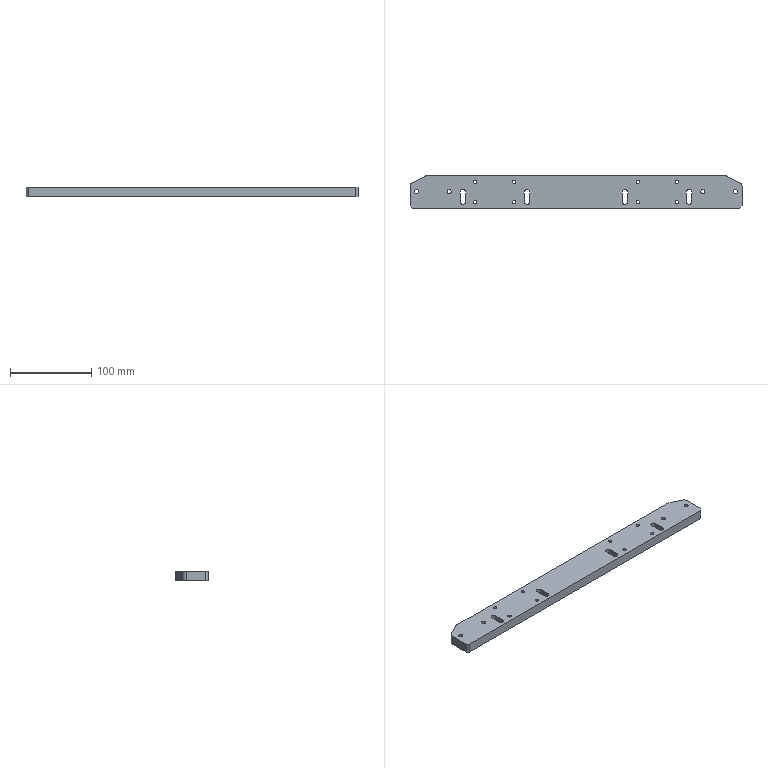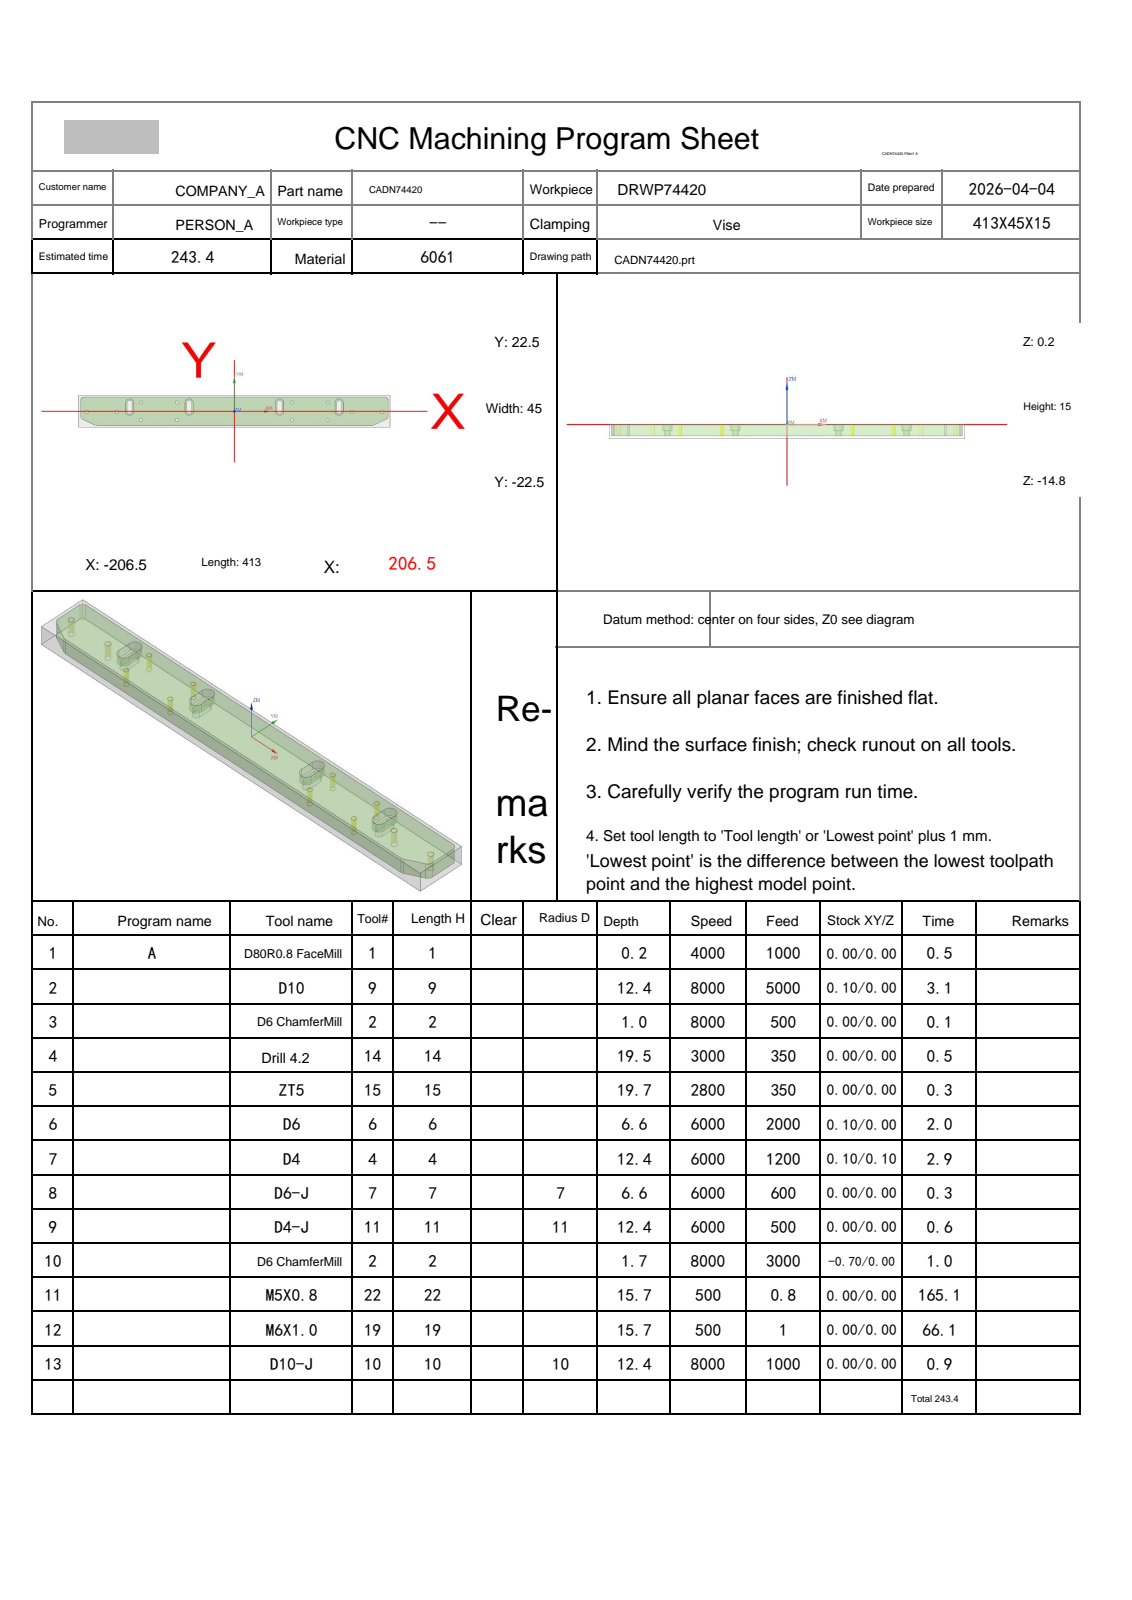NC program | NX | posted by the shop | part box 408 x 40 x 12 mm
Lines 1072 to 2398 of 2398:
N7 T04 M06
(D4  D=4. R=0. H=04 ce=0.10 di=0.10)
G00 G90 G54 X-140.2 Y6. M03 S6000
G43 H04 Z20.
M08
Z-5.9
G01 Y0.0 Z-5.946 F1200.
G03 X-139. Y-1.2 Z-5.961 I1.2 J0.0
X-137.8 Y0.0 Z-5.975 I0.0 J1.2
G01 Y12. Z-6.067
G03 X-139. Y13.2 Z-6.082 I-1.2 J0.0
X-140.2 Y12. Z-6.096 I0.0 J-1.2
G01 Y0.0 Z-6.188
G03 X-139. Y-1.2 Z-6.203 I1.2 J0.0
X-137.8 Y0.0 Z-6.217 I0.0 J1.2
G01 Y12. Z-6.31
G03 X-139. Y13.2 Z-6.324 I-1.2 J0.0
X-140.2 Y12. Z-6.339 I0.0 J-1.2
G01 Y0.0 Z-6.431
G03 X-139. Y-1.2 Z-6.445 I1.2 J0.0
X-137.8 Y0.0 Z-6.46 I0.0 J1.2
G01 Y12. Z-6.552
G03 X-139. Y13.2 Z-6.566 I-1.2 J0.0
X-140.2 Y12. Z-6.581 I0.0 J-1.2
G01 Y0.0 Z-6.673
G03 X-139. Y-1.2 Z-6.688 I1.2 J0.0
X-137.8 Y0.0 Z-6.702 I0.0 J1.2
G01 Y12. Z-6.794
G03 X-139. Y13.2 Z-6.809 I-1.2 J0.0
X-140.2 Y12. Z-6.823 I0.0 J-1.2
G01 Y0.0 Z-6.915
G03 X-139. Y-1.2 Z-6.93 I1.2 J0.0
X-137.8 Y0.0 Z-6.944 I0.0 J1.2
G01 Y12. Z-7.036
G03 X-139. Y13.2 Z-7.051 I-1.2 J0.0
X-140.2 Y12. Z-7.065 I0.0 J-1.2
G01 Y0.0 Z-7.158
G03 X-139. Y-1.2 Z-7.172 I1.2 J0.0
X-137.8 Y0.0 Z-7.187 I0.0 J1.2
G01 Y12. Z-7.279
G03 X-139. Y13.2 Z-7.293 I-1.2 J0.0
X-140.2 Y12. Z-7.308 I0.0 J-1.2
G01 Y0.0 Z-7.4
G03 X-139. Y-1.2 Z-7.414 I1.2 J0.0
X-137.8 Y0.0 Z-7.429 I0.0 J1.2
G01 Y12. Z-7.521
G03 X-139. Y13.2 Z-7.536 I-1.2 J0.0
X-140.2 Y12. Z-7.55 I0.0 J-1.2
G01 Y0.0 Z-7.642
G03 X-139. Y-1.2 Z-7.657 I1.2 J0.0
X-137.8 Y0.0 Z-7.671 I0.0 J1.2
G01 Y12. Z-7.763
G03 X-139. Y13.2 Z-7.778 I-1.2 J0.0
X-140.2 Y12. Z-7.792 I0.0 J-1.2
G01 Y0.0 Z-7.885
G03 X-139. Y-1.2 Z-7.899 I1.2 J0.0
X-137.8 Y0.0 Z-7.914 I0.0 J1.2
G01 Y12. Z-8.006
G03 X-139. Y13.2 Z-8.02 I-1.2 J0.0
X-140.2 Y12. Z-8.035 I0.0 J-1.2
G01 Y0.0 Z-8.127
G03 X-139. Y-1.2 Z-8.141 I1.2 J0.0
X-137.8 Y0.0 Z-8.156 I0.0 J1.2
G01 Y12. Z-8.248
G03 X-139. Y13.2 Z-8.263 I-1.2 J0.0
X-140.2 Y12. Z-8.277 I0.0 J-1.2
G01 Y0.0 Z-8.369
G03 X-139. Y-1.2 Z-8.384 I1.2 J0.0
X-137.8 Y0.0 Z-8.398 I0.0 J1.2
G01 Y12. Z-8.49
G03 X-139. Y13.2 Z-8.505 I-1.2 J0.0
X-140.2 Y12. Z-8.519 I0.0 J-1.2
G01 Y0.0 Z-8.611
G03 X-139. Y-1.2 Z-8.626 I1.2 J0.0
X-137.8 Y0.0 Z-8.64 I0.0 J1.2
G01 Y12. Z-8.733
G03 X-139. Y13.2 Z-8.747 I-1.2 J0.0
X-140.2 Y12. Z-8.762 I0.0 J-1.2
G01 Y0.0 Z-8.854
G03 X-139. Y-1.2 Z-8.868 I1.2 J0.0
X-137.8 Y0.0 Z-8.883 I0.0 J1.2
G01 Y12. Z-8.975
G03 X-139. Y13.2 Z-8.989 I-1.2 J0.0
X-140.2 Y12. Z-9.004 I0.0 J-1.2
G01 Y0.0 Z-9.096
G03 X-139. Y-1.2 Z-9.111 I1.2 J0.0
X-137.8 Y0.0 Z-9.125 I0.0 J1.2
G01 Y12. Z-9.217
G03 X-139. Y13.2 Z-9.232 I-1.2 J0.0
X-140.2 Y12. Z-9.246 I0.0 J-1.2
G01 Y0.0 Z-9.338
G03 X-139. Y-1.2 Z-9.353 I1.2 J0.0
X-137.8 Y0.0 Z-9.367 I0.0 J1.2
G01 Y12. Z-9.46
G03 X-139. Y13.2 Z-9.474 I-1.2 J0.0
X-140.2 Y12. Z-9.489 I0.0 J-1.2
G01 Y0.0 Z-9.581
G03 X-139. Y-1.2 Z-9.595 I1.2 J0.0
X-137.8 Y0.0 Z-9.61 I0.0 J1.2
G01 Y12. Z-9.702
G03 X-139. Y13.2 Z-9.716 I-1.2 J0.0
X-140.2 Y12. Z-9.731 I0.0 J-1.2
G01 Y0.0 Z-9.823
G03 X-139. Y-1.2 Z-9.838 I1.2 J0.0
X-137.8 Y0.0 Z-9.852 I0.0 J1.2
G01 Y12. Z-9.944
G03 X-139. Y13.2 Z-9.959 I-1.2 J0.0
X-140.2 Y12. Z-9.973 I0.0 J-1.2
G01 Y0.0 Z-10.065
G03 X-139. Y-1.2 Z-10.08 I1.2 J0.0
X-137.8 Y0.0 Z-10.094 I0.0 J1.2
G01 Y12. Z-10.186
G03 X-139. Y13.2 Z-10.201 I-1.2 J0.0
X-140.2 Y12. Z-10.215 I0.0 J-1.2
G01 Y0.0 Z-10.308
G03 X-139. Y-1.2 Z-10.322 I1.2 J0.0
X-137.8 Y0.0 Z-10.337 I0.0 J1.2
G01 Y12. Z-10.429
G03 X-139. Y13.2 Z-10.443 I-1.2 J0.0
X-140.2 Y12. Z-10.458 I0.0 J-1.2
G01 Y0.0 Z-10.55
G03 X-139. Y-1.2 Z-10.564 I1.2 J0.0
X-137.8 Y0.0 Z-10.579 I0.0 J1.2
G01 Y12. Z-10.671
G03 X-139. Y13.2 Z-10.686 I-1.2 J0.0
X-140.2 Y12. Z-10.7 I0.0 J-1.2
G01 Y0.0 Z-10.792
G03 X-139. Y-1.2 Z-10.807 I1.2 J0.0
X-137.8 Y0.0 Z-10.821 I0.0 J1.2
G01 Y12. Z-10.913
G03 X-139. Y13.2 Z-10.928 I-1.2 J0.0
X-140.2 Y12. Z-10.942 I0.0 J-1.2
G01 Y0.0 Z-11.035
G03 X-139. Y-1.2 Z-11.049 I1.2 J0.0
X-137.8 Y0.0 Z-11.064 I0.0 J1.2
G01 Y12. Z-11.156
G03 X-139. Y13.2 Z-11.17 I-1.2 J0.0
X-140.2 Y12. Z-11.185 I0.0 J-1.2
G01 Y0.0 Z-11.277
G03 X-139. Y-1.2 Z-11.291 I1.2 J0.0
X-137.8 Y0.0 Z-11.306 I0.0 J1.2
G01 Y12. Z-11.398
G03 X-139. Y13.2 Z-11.413 I-1.2 J0.0
X-140.2 Y12. Z-11.427 I0.0 J-1.2
G01 Y0.0 Z-11.519
G03 X-139. Y-1.2 Z-11.534 I1.2 J0.0
X-137.8 Y0.0 Z-11.548 I0.0 J1.2
G01 Y12. Z-11.64
G03 X-139. Y13.2 Z-11.655 I-1.2 J0.0
X-140.2 Y12. Z-11.669 I0.0 J-1.2
G01 Y0.0 Z-11.761
G03 X-139. Y-1.2 Z-11.776 I1.2 J0.0
X-137.8 Y0.0 Z-11.79 I0.0 J1.2
G01 Y12. Z-11.883
G03 X-139. Y13.2 Z-11.897 I-1.2 J0.0
X-140.2 Y12. Z-11.912 I0.0 J-1.2
G01 Y0.0 Z-12.004
G03 X-139. Y-1.2 Z-12.018 I1.2 J0.0
X-137.8 Y0.0 Z-12.033 I0.0 J1.2
G01 Y12. Z-12.125
G03 X-139. Y13.2 Z-12.139 I-1.2 J0.0
X-140.2 Y12. Z-12.154 I0.0 J-1.2
G01 Y6. Z-12.2
Y0.0
G03 X-139. Y-1.2 I1.2 J0.0
X-137.8 Y0.0 I0.0 J1.2
G01 Y12.
G03 X-139. Y13.2 I-1.2 J0.0
X-140.2 Y12. I0.0 J-1.2
G01 Y6.
Y5.5
Z-11.2
G00 Z20.
X-61.2 Y6.
Z-5.9
G01 Y0.0 Z-5.946
G03 X-60. Y-1.2 Z-5.961 I1.2 J0.0
X-58.8 Y0.0 Z-5.975 I0.0 J1.2
G01 Y12. Z-6.067
G03 X-59.28 Y12.96 Z-6.076 I-1.2 J0.0
X-60. Y13.2 Z-6.082 I-.72 J-.96
X-61.2 Y12. Z-6.096 I0.0 J-1.2
G01 Y0.0 Z-6.188
G03 X-60. Y-1.2 Z-6.203 I1.2 J0.0
X-58.8 Y0.0 Z-6.217 I0.0 J1.2
G01 Y12. Z-6.31
G03 X-59.28 Y12.96 Z-6.318 I-1.2 J0.0
X-60. Y13.2 Z-6.324 I-.72 J-.96
X-61.2 Y12. Z-6.339 I0.0 J-1.2
G01 Y0.0 Z-6.431
G03 X-60. Y-1.2 Z-6.445 I1.2 J0.0
X-58.8 Y0.0 Z-6.46 I0.0 J1.2
G01 Y12. Z-6.552
G03 X-59.28 Y12.96 Z-6.56 I-1.2 J0.0
X-60. Y13.2 Z-6.566 I-.72 J-.96
X-61.2 Y12. Z-6.581 I0.0 J-1.2
G01 Y0.0 Z-6.673
G03 X-60. Y-1.2 Z-6.688 I1.2 J0.0
X-58.8 Y0.0 Z-6.702 I0.0 J1.2
G01 Y12. Z-6.794
G03 X-59.28 Y12.96 Z-6.803 I-1.2 J0.0
X-60. Y13.2 Z-6.809 I-.72 J-.96
X-61.2 Y12. Z-6.823 I0.0 J-1.2
G01 Y0.0 Z-6.915
G03 X-60. Y-1.2 Z-6.93 I1.2 J0.0
X-58.8 Y0.0 Z-6.944 I0.0 J1.2
G01 Y12. Z-7.036
G03 X-59.28 Y12.96 Z-7.045 I-1.2 J0.0
X-60. Y13.2 Z-7.051 I-.72 J-.96
X-61.2 Y12. Z-7.065 I0.0 J-1.2
G01 Y0.0 Z-7.158
G03 X-60. Y-1.2 Z-7.172 I1.2 J0.0
X-58.8 Y0.0 Z-7.187 I0.0 J1.2
G01 Y12. Z-7.279
G03 X-59.28 Y12.96 Z-7.287 I-1.2 J0.0
X-60. Y13.2 Z-7.293 I-.72 J-.96
X-61.2 Y12. Z-7.308 I0.0 J-1.2
G01 Y0.0 Z-7.4
G03 X-60. Y-1.2 Z-7.414 I1.2 J0.0
X-58.8 Y0.0 Z-7.429 I0.0 J1.2
G01 Y12. Z-7.521
G03 X-59.28 Y12.96 Z-7.53 I-1.2 J0.0
X-60. Y13.2 Z-7.536 I-.72 J-.96
X-61.2 Y12. Z-7.55 I0.0 J-1.2
G01 Y0.0 Z-7.642
G03 X-60. Y-1.2 Z-7.657 I1.2 J0.0
X-58.8 Y0.0 Z-7.671 I0.0 J1.2
G01 Y12. Z-7.763
G03 X-59.28 Y12.96 Z-7.772 I-1.2 J0.0
X-60. Y13.2 Z-7.778 I-.72 J-.96
X-61.2 Y12. Z-7.792 I0.0 J-1.2
G01 Y0.0 Z-7.885
G03 X-60. Y-1.2 Z-7.899 I1.2 J0.0
X-58.8 Y0.0 Z-7.914 I0.0 J1.2
G01 Y12. Z-8.006
G03 X-59.28 Y12.96 Z-8.014 I-1.2 J0.0
X-60. Y13.2 Z-8.02 I-.72 J-.96
X-61.2 Y12. Z-8.035 I0.0 J-1.2
G01 Y0.0 Z-8.127
G03 X-60. Y-1.2 Z-8.141 I1.2 J0.0
X-58.8 Y0.0 Z-8.156 I0.0 J1.2
G01 Y12. Z-8.248
G03 X-59.28 Y12.96 Z-8.257 I-1.2 J0.0
X-60. Y13.2 Z-8.263 I-.72 J-.96
X-61.2 Y12. Z-8.277 I0.0 J-1.2
G01 Y0.0 Z-8.369
G03 X-60. Y-1.2 Z-8.384 I1.2 J0.0
X-58.8 Y0.0 Z-8.398 I0.0 J1.2
G01 Y12. Z-8.49
G03 X-59.28 Y12.96 Z-8.499 I-1.2 J0.0
X-60. Y13.2 Z-8.505 I-.72 J-.96
X-61.2 Y12. Z-8.519 I0.0 J-1.2
G01 Y0.0 Z-8.611
G03 X-60. Y-1.2 Z-8.626 I1.2 J0.0
X-58.8 Y0.0 Z-8.64 I0.0 J1.2
G01 Y12. Z-8.733
G03 X-59.28 Y12.96 Z-8.741 I-1.2 J0.0
X-60. Y13.2 Z-8.747 I-.72 J-.96
X-61.2 Y12. Z-8.762 I0.0 J-1.2
G01 Y0.0 Z-8.854
G03 X-60. Y-1.2 Z-8.868 I1.2 J0.0
X-58.8 Y0.0 Z-8.883 I0.0 J1.2
G01 Y12. Z-8.975
G03 X-59.28 Y12.96 Z-8.983 I-1.2 J0.0
X-60. Y13.2 Z-8.989 I-.72 J-.96
X-61.2 Y12. Z-9.004 I0.0 J-1.2
G01 Y0.0 Z-9.096
G03 X-60. Y-1.2 Z-9.111 I1.2 J0.0
X-58.8 Y0.0 Z-9.125 I0.0 J1.2
G01 Y12. Z-9.217
G03 X-59.28 Y12.96 Z-9.226 I-1.2 J0.0
X-60. Y13.2 Z-9.232 I-.72 J-.96
X-61.2 Y12. Z-9.246 I0.0 J-1.2
G01 Y0.0 Z-9.338
G03 X-60. Y-1.2 Z-9.353 I1.2 J0.0
X-58.8 Y0.0 Z-9.367 I0.0 J1.2
G01 Y12. Z-9.46
G03 X-59.28 Y12.96 Z-9.468 I-1.2 J0.0
X-60. Y13.2 Z-9.474 I-.72 J-.96
X-61.2 Y12. Z-9.489 I0.0 J-1.2
G01 Y0.0 Z-9.581
G03 X-60. Y-1.2 Z-9.595 I1.2 J0.0
X-58.8 Y0.0 Z-9.61 I0.0 J1.2
G01 Y12. Z-9.702
G03 X-59.28 Y12.96 Z-9.71 I-1.2 J0.0
X-60. Y13.2 Z-9.716 I-.72 J-.96
X-61.2 Y12. Z-9.731 I0.0 J-1.2
G01 Y0.0 Z-9.823
G03 X-60. Y-1.2 Z-9.838 I1.2 J0.0
X-58.8 Y0.0 Z-9.852 I0.0 J1.2
G01 Y12. Z-9.944
G03 X-59.28 Y12.96 Z-9.953 I-1.2 J0.0
X-60. Y13.2 Z-9.959 I-.72 J-.96
X-61.2 Y12. Z-9.973 I0.0 J-1.2
G01 Y0.0 Z-10.065
G03 X-60. Y-1.2 Z-10.08 I1.2 J0.0
X-58.8 Y0.0 Z-10.094 I0.0 J1.2
G01 Y12. Z-10.186
G03 X-59.28 Y12.96 Z-10.195 I-1.2 J0.0
X-60. Y13.2 Z-10.201 I-.72 J-.96
X-61.2 Y12. Z-10.215 I0.0 J-1.2
G01 Y0.0 Z-10.308
G03 X-60. Y-1.2 Z-10.322 I1.2 J0.0
X-58.8 Y0.0 Z-10.337 I0.0 J1.2
G01 Y12. Z-10.429
G03 X-59.28 Y12.96 Z-10.437 I-1.2 J0.0
X-60. Y13.2 Z-10.443 I-.72 J-.96
X-61.2 Y12. Z-10.458 I0.0 J-1.2
G01 Y0.0 Z-10.55
G03 X-60. Y-1.2 Z-10.564 I1.2 J0.0
X-58.8 Y0.0 Z-10.579 I0.0 J1.2
G01 Y12. Z-10.671
G03 X-59.28 Y12.96 Z-10.68 I-1.2 J0.0
X-60. Y13.2 Z-10.686 I-.72 J-.96
X-61.2 Y12. Z-10.7 I0.0 J-1.2
G01 Y0.0 Z-10.792
G03 X-60. Y-1.2 Z-10.807 I1.2 J0.0
X-58.8 Y0.0 Z-10.821 I0.0 J1.2
G01 Y12. Z-10.913
G03 X-59.28 Y12.96 Z-10.922 I-1.2 J0.0
X-60. Y13.2 Z-10.928 I-.72 J-.96
X-61.2 Y12. Z-10.942 I0.0 J-1.2
G01 Y0.0 Z-11.035
G03 X-60. Y-1.2 Z-11.049 I1.2 J0.0
X-58.8 Y0.0 Z-11.064 I0.0 J1.2
G01 Y12. Z-11.156
G03 X-59.28 Y12.96 Z-11.164 I-1.2 J0.0
X-60. Y13.2 Z-11.17 I-.72 J-.96
X-61.2 Y12. Z-11.185 I0.0 J-1.2
G01 Y0.0 Z-11.277
G03 X-60. Y-1.2 Z-11.291 I1.2 J0.0
X-58.8 Y0.0 Z-11.306 I0.0 J1.2
G01 Y12. Z-11.398
G03 X-59.28 Y12.96 Z-11.407 I-1.2 J0.0
X-60. Y13.2 Z-11.413 I-.72 J-.96
X-61.2 Y12. Z-11.427 I0.0 J-1.2
G01 Y0.0 Z-11.519
G03 X-60. Y-1.2 Z-11.534 I1.2 J0.0
X-58.8 Y0.0 Z-11.548 I0.0 J1.2
G01 Y12. Z-11.64
G03 X-59.28 Y12.96 Z-11.649 I-1.2 J0.0
X-60. Y13.2 Z-11.655 I-.72 J-.96
X-61.2 Y12. Z-11.669 I0.0 J-1.2
G01 Y0.0 Z-11.761
G03 X-60. Y-1.2 Z-11.776 I1.2 J0.0
X-58.8 Y0.0 Z-11.79 I0.0 J1.2
G01 Y12. Z-11.883
G03 X-59.28 Y12.96 Z-11.891 I-1.2 J0.0
X-60. Y13.2 Z-11.897 I-.72 J-.96
X-61.2 Y12. Z-11.912 I0.0 J-1.2
G01 Y0.0 Z-12.004
G03 X-60. Y-1.2 Z-12.018 I1.2 J0.0
X-58.8 Y0.0 Z-12.033 I0.0 J1.2
G01 Y12. Z-12.125
G03 X-59.28 Y12.96 Z-12.133 I-1.2 J0.0
X-60. Y13.2 Z-12.139 I-.72 J-.96
X-61.2 Y12. Z-12.154 I0.0 J-1.2
G01 Y6. Z-12.2
Y0.0
G03 X-60. Y-1.2 I1.2 J0.0
X-58.8 Y0.0 I0.0 J1.2
G01 Y12.
G03 X-60. Y13.2 I-1.2 J0.0
X-61.2 Y12. I0.0 J-1.2
G01 Y6.
Y5.5
Z-11.2
G00 Z20.
X58.8 Y6.
Z-5.9
G01 Y0.0 Z-5.946
G03 X60. Y-1.2 Z-5.961 I1.2 J0.0
X61.2 Y0.0 Z-5.975 I0.0 J1.2
G01 Y12. Z-6.067
G03 X60. Y13.2 Z-6.082 I-1.2 J0.0
X59.316 Y12.986 Z-6.087 I0.0 J-1.2
X58.8 Y12. Z-6.096 I.684 J-.986
G01 Y0.0 Z-6.188
G03 X60. Y-1.2 Z-6.203 I1.2 J0.0
X61.2 Y0.0 Z-6.217 I0.0 J1.2
G01 Y12. Z-6.31
G03 X60. Y13.2 Z-6.324 I-1.2 J0.0
X59.316 Y12.986 Z-6.33 I0.0 J-1.2
X58.8 Y12. Z-6.339 I.684 J-.986
G01 Y0.0 Z-6.431
G03 X60. Y-1.2 Z-6.445 I1.2 J0.0
X61.2 Y0.0 Z-6.46 I0.0 J1.2
G01 Y12. Z-6.552
G03 X60. Y13.2 Z-6.566 I-1.2 J0.0
X59.316 Y12.986 Z-6.572 I0.0 J-1.2
X58.8 Y12. Z-6.581 I.684 J-.986
G01 Y0.0 Z-6.673
G03 X60. Y-1.2 Z-6.688 I1.2 J0.0
X61.2 Y0.0 Z-6.702 I0.0 J1.2
G01 Y12. Z-6.794
G03 X60. Y13.2 Z-6.809 I-1.2 J0.0
X59.316 Y12.986 Z-6.814 I0.0 J-1.2
X58.8 Y12. Z-6.823 I.684 J-.986
G01 Y0.0 Z-6.915
G03 X60. Y-1.2 Z-6.93 I1.2 J0.0
X61.2 Y0.0 Z-6.944 I0.0 J1.2
G01 Y12. Z-7.036
G03 X60. Y13.2 Z-7.051 I-1.2 J0.0
X59.316 Y12.986 Z-7.057 I0.0 J-1.2
X58.8 Y12. Z-7.065 I.684 J-.986
G01 Y0.0 Z-7.158
G03 X60. Y-1.2 Z-7.172 I1.2 J0.0
X61.2 Y0.0 Z-7.187 I0.0 J1.2
G01 Y12. Z-7.279
G03 X60. Y13.2 Z-7.293 I-1.2 J0.0
X59.316 Y12.986 Z-7.299 I0.0 J-1.2
X58.8 Y12. Z-7.308 I.684 J-.986
G01 Y0.0 Z-7.4
G03 X60. Y-1.2 Z-7.414 I1.2 J0.0
X61.2 Y0.0 Z-7.429 I0.0 J1.2
G01 Y12. Z-7.521
G03 X60. Y13.2 Z-7.536 I-1.2 J0.0
X59.316 Y12.986 Z-7.541 I0.0 J-1.2
X58.8 Y12. Z-7.55 I.684 J-.986
G01 Y0.0 Z-7.642
G03 X60. Y-1.2 Z-7.657 I1.2 J0.0
X61.2 Y0.0 Z-7.671 I0.0 J1.2
G01 Y12. Z-7.763
G03 X60. Y13.2 Z-7.778 I-1.2 J0.0
X59.316 Y12.986 Z-7.783 I0.0 J-1.2
X58.8 Y12. Z-7.792 I.684 J-.986
G01 Y0.0 Z-7.885
G03 X60. Y-1.2 Z-7.899 I1.2 J0.0
X61.2 Y0.0 Z-7.914 I0.0 J1.2
G01 Y12. Z-8.006
G03 X60. Y13.2 Z-8.02 I-1.2 J0.0
X59.316 Y12.986 Z-8.026 I0.0 J-1.2
X58.8 Y12. Z-8.035 I.684 J-.986
G01 Y0.0 Z-8.127
G03 X60. Y-1.2 Z-8.141 I1.2 J0.0
X61.2 Y0.0 Z-8.156 I0.0 J1.2
G01 Y12. Z-8.248
G03 X60. Y13.2 Z-8.263 I-1.2 J0.0
X59.316 Y12.986 Z-8.268 I0.0 J-1.2
X58.8 Y12. Z-8.277 I.684 J-.986
G01 Y0.0 Z-8.369
G03 X60. Y-1.2 Z-8.384 I1.2 J0.0
X61.2 Y0.0 Z-8.398 I0.0 J1.2
G01 Y12. Z-8.49
G03 X60. Y13.2 Z-8.505 I-1.2 J0.0
X59.316 Y12.986 Z-8.51 I0.0 J-1.2
X58.8 Y12. Z-8.519 I.684 J-.986
G01 Y0.0 Z-8.611
G03 X60. Y-1.2 Z-8.626 I1.2 J0.0
X61.2 Y0.0 Z-8.64 I0.0 J1.2
G01 Y12. Z-8.733
G03 X60. Y13.2 Z-8.747 I-1.2 J0.0
X59.316 Y12.986 Z-8.753 I0.0 J-1.2
X58.8 Y12. Z-8.762 I.684 J-.986
G01 Y0.0 Z-8.854
G03 X60. Y-1.2 Z-8.868 I1.2 J0.0
X61.2 Y0.0 Z-8.883 I0.0 J1.2
G01 Y12. Z-8.975
G03 X60. Y13.2 Z-8.989 I-1.2 J0.0
X59.316 Y12.986 Z-8.995 I0.0 J-1.2
X58.8 Y12. Z-9.004 I.684 J-.986
G01 Y0.0 Z-9.096
G03 X60. Y-1.2 Z-9.111 I1.2 J0.0
X61.2 Y0.0 Z-9.125 I0.0 J1.2
G01 Y12. Z-9.217
G03 X60. Y13.2 Z-9.232 I-1.2 J0.0
X59.316 Y12.986 Z-9.237 I0.0 J-1.2
X58.8 Y12. Z-9.246 I.684 J-.986
G01 Y0.0 Z-9.338
G03 X60. Y-1.2 Z-9.353 I1.2 J0.0
X61.2 Y0.0 Z-9.367 I0.0 J1.2
G01 Y12. Z-9.46
G03 X60. Y13.2 Z-9.474 I-1.2 J0.0
X59.316 Y12.986 Z-9.48 I0.0 J-1.2
X58.8 Y12. Z-9.489 I.684 J-.986
G01 Y0.0 Z-9.581
G03 X60. Y-1.2 Z-9.595 I1.2 J0.0
X61.2 Y0.0 Z-9.61 I0.0 J1.2
G01 Y12. Z-9.702
G03 X60. Y13.2 Z-9.716 I-1.2 J0.0
X59.316 Y12.986 Z-9.722 I0.0 J-1.2
X58.8 Y12. Z-9.731 I.684 J-.986
G01 Y0.0 Z-9.823
G03 X60. Y-1.2 Z-9.838 I1.2 J0.0
X61.2 Y0.0 Z-9.852 I0.0 J1.2
G01 Y12. Z-9.944
G03 X60. Y13.2 Z-9.959 I-1.2 J0.0
X59.316 Y12.986 Z-9.964 I0.0 J-1.2
X58.8 Y12. Z-9.973 I.684 J-.986
G01 Y0.0 Z-10.065
G03 X60. Y-1.2 Z-10.08 I1.2 J0.0
X61.2 Y0.0 Z-10.094 I0.0 J1.2
G01 Y12. Z-10.186
G03 X60. Y13.2 Z-10.201 I-1.2 J0.0
X59.316 Y12.986 Z-10.207 I0.0 J-1.2
X58.8 Y12. Z-10.215 I.684 J-.986
G01 Y0.0 Z-10.308
G03 X60. Y-1.2 Z-10.322 I1.2 J0.0
X61.2 Y0.0 Z-10.337 I0.0 J1.2
G01 Y12. Z-10.429
G03 X60. Y13.2 Z-10.443 I-1.2 J0.0
X59.316 Y12.986 Z-10.449 I0.0 J-1.2
X58.8 Y12. Z-10.458 I.684 J-.986
G01 Y0.0 Z-10.55
G03 X60. Y-1.2 Z-10.564 I1.2 J0.0
X61.2 Y0.0 Z-10.579 I0.0 J1.2
G01 Y12. Z-10.671
G03 X60. Y13.2 Z-10.686 I-1.2 J0.0
X59.316 Y12.986 Z-10.691 I0.0 J-1.2
X58.8 Y12. Z-10.7 I.684 J-.986
G01 Y0.0 Z-10.792
G03 X60. Y-1.2 Z-10.807 I1.2 J0.0
X61.2 Y0.0 Z-10.821 I0.0 J1.2
G01 Y12. Z-10.913
G03 X60. Y13.2 Z-10.928 I-1.2 J0.0
X59.316 Y12.986 Z-10.933 I0.0 J-1.2
X58.8 Y12. Z-10.942 I.684 J-.986
G01 Y0.0 Z-11.035
G03 X60. Y-1.2 Z-11.049 I1.2 J0.0
X61.2 Y0.0 Z-11.064 I0.0 J1.2
G01 Y12. Z-11.156
G03 X60. Y13.2 Z-11.17 I-1.2 J0.0
X59.316 Y12.986 Z-11.176 I0.0 J-1.2
X58.8 Y12. Z-11.185 I.684 J-.986
G01 Y0.0 Z-11.277
G03 X60. Y-1.2 Z-11.291 I1.2 J0.0
X61.2 Y0.0 Z-11.306 I0.0 J1.2
G01 Y12. Z-11.398
G03 X60. Y13.2 Z-11.413 I-1.2 J0.0
X59.316 Y12.986 Z-11.418 I0.0 J-1.2
X58.8 Y12. Z-11.427 I.684 J-.986
G01 Y0.0 Z-11.519
G03 X60. Y-1.2 Z-11.534 I1.2 J0.0
X61.2 Y0.0 Z-11.548 I0.0 J1.2
G01 Y12. Z-11.64
G03 X60. Y13.2 Z-11.655 I-1.2 J0.0
X59.316 Y12.986 Z-11.66 I0.0 J-1.2
X58.8 Y12. Z-11.669 I.684 J-.986
G01 Y0.0 Z-11.761
G03 X60. Y-1.2 Z-11.776 I1.2 J0.0
X61.2 Y0.0 Z-11.79 I0.0 J1.2
G01 Y12. Z-11.883
G03 X60. Y13.2 Z-11.897 I-1.2 J0.0
X59.316 Y12.986 Z-11.903 I0.0 J-1.2
X58.8 Y12. Z-11.912 I.684 J-.986
G01 Y0.0 Z-12.004
G03 X60. Y-1.2 Z-12.018 I1.2 J0.0
X61.2 Y0.0 Z-12.033 I0.0 J1.2
G01 Y12. Z-12.125
G03 X60. Y13.2 Z-12.139 I-1.2 J0.0
X59.316 Y12.986 Z-12.145 I0.0 J-1.2
X58.8 Y12. Z-12.154 I.684 J-.986
G01 Y6. Z-12.2
Y0.0
G03 X60. Y-1.2 I1.2 J0.0
X61.2 Y0.0 I0.0 J1.2
G01 Y12.
G03 X60. Y13.2 I-1.2 J0.0
X58.8 Y12. I0.0 J-1.2
G01 Y6.
Y5.5
Z-11.2
G00 Z20.
X137.8 Y6.
Z-5.9
G01 Y0.0 Z-5.946
G03 X139. Y-1.2 Z-5.961 I1.2 J0.0
X140.2 Y0.0 Z-5.975 I0.0 J1.2
G01 Y12. Z-6.067
G03 X139. Y13.2 Z-6.082 I-1.2 J0.0
X137.8 Y12. Z-6.096 I0.0 J-1.2
G01 Y0.0 Z-6.188
G03 X139. Y-1.2 Z-6.203 I1.2 J0.0
X140.2 Y0.0 Z-6.217 I0.0 J1.2
G01 Y12. Z-6.31
G03 X139. Y13.2 Z-6.324 I-1.2 J0.0
X137.8 Y12. Z-6.339 I0.0 J-1.2
G01 Y0.0 Z-6.431
G03 X139. Y-1.2 Z-6.445 I1.2 J0.0
X140.2 Y0.0 Z-6.46 I0.0 J1.2
G01 Y12. Z-6.552
G03 X139. Y13.2 Z-6.566 I-1.2 J0.0
X137.8 Y12. Z-6.581 I0.0 J-1.2
G01 Y0.0 Z-6.673
G03 X139. Y-1.2 Z-6.688 I1.2 J0.0
X140.2 Y0.0 Z-6.702 I0.0 J1.2
G01 Y12. Z-6.794
G03 X139. Y13.2 Z-6.809 I-1.2 J0.0
X137.8 Y12. Z-6.823 I0.0 J-1.2
G01 Y0.0 Z-6.915
G03 X139. Y-1.2 Z-6.93 I1.2 J0.0
X140.2 Y0.0 Z-6.944 I0.0 J1.2
G01 Y12. Z-7.036
G03 X139. Y13.2 Z-7.051 I-1.2 J0.0
X137.8 Y12. Z-7.065 I0.0 J-1.2
G01 Y0.0 Z-7.158
G03 X139. Y-1.2 Z-7.172 I1.2 J0.0
X140.2 Y0.0 Z-7.187 I0.0 J1.2
G01 Y12. Z-7.279
G03 X139. Y13.2 Z-7.293 I-1.2 J0.0
X137.8 Y12. Z-7.308 I0.0 J-1.2
G01 Y0.0 Z-7.4
G03 X139. Y-1.2 Z-7.414 I1.2 J0.0
X140.2 Y0.0 Z-7.429 I0.0 J1.2
G01 Y12. Z-7.521
G03 X139. Y13.2 Z-7.536 I-1.2 J0.0
X137.8 Y12. Z-7.55 I0.0 J-1.2
G01 Y0.0 Z-7.642
G03 X139. Y-1.2 Z-7.657 I1.2 J0.0
X140.2 Y0.0 Z-7.671 I0.0 J1.2
G01 Y12. Z-7.763
G03 X139. Y13.2 Z-7.778 I-1.2 J0.0
X137.8 Y12. Z-7.792 I0.0 J-1.2
G01 Y0.0 Z-7.885
G03 X139. Y-1.2 Z-7.899 I1.2 J0.0
X140.2 Y0.0 Z-7.914 I0.0 J1.2
G01 Y12. Z-8.006
G03 X139. Y13.2 Z-8.02 I-1.2 J0.0
X137.8 Y12. Z-8.035 I0.0 J-1.2
G01 Y0.0 Z-8.127
G03 X139. Y-1.2 Z-8.141 I1.2 J0.0
X140.2 Y0.0 Z-8.156 I0.0 J1.2
G01 Y12. Z-8.248
G03 X139. Y13.2 Z-8.263 I-1.2 J0.0
X137.8 Y12. Z-8.277 I0.0 J-1.2
G01 Y0.0 Z-8.369
G03 X139. Y-1.2 Z-8.384 I1.2 J0.0
X140.2 Y0.0 Z-8.398 I0.0 J1.2
G01 Y12. Z-8.49
G03 X139. Y13.2 Z-8.505 I-1.2 J0.0
X137.8 Y12. Z-8.519 I0.0 J-1.2
G01 Y0.0 Z-8.611
G03 X139. Y-1.2 Z-8.626 I1.2 J0.0
X140.2 Y0.0 Z-8.64 I0.0 J1.2
G01 Y12. Z-8.733
G03 X139. Y13.2 Z-8.747 I-1.2 J0.0
X137.8 Y12. Z-8.762 I0.0 J-1.2
G01 Y0.0 Z-8.854
G03 X139. Y-1.2 Z-8.868 I1.2 J0.0
X140.2 Y0.0 Z-8.883 I0.0 J1.2
G01 Y12. Z-8.975
G03 X139. Y13.2 Z-8.989 I-1.2 J0.0
X137.8 Y12. Z-9.004 I0.0 J-1.2
G01 Y0.0 Z-9.096
G03 X139. Y-1.2 Z-9.111 I1.2 J0.0
X140.2 Y0.0 Z-9.125 I0.0 J1.2
G01 Y12. Z-9.217
G03 X139. Y13.2 Z-9.232 I-1.2 J0.0
X137.8 Y12. Z-9.246 I0.0 J-1.2
G01 Y0.0 Z-9.338
G03 X139. Y-1.2 Z-9.353 I1.2 J0.0
X140.2 Y0.0 Z-9.367 I0.0 J1.2
G01 Y12. Z-9.46
G03 X139. Y13.2 Z-9.474 I-1.2 J0.0
X137.8 Y12. Z-9.489 I0.0 J-1.2
G01 Y0.0 Z-9.581
G03 X139. Y-1.2 Z-9.595 I1.2 J0.0
X140.2 Y0.0 Z-9.61 I0.0 J1.2
G01 Y12. Z-9.702
G03 X139. Y13.2 Z-9.716 I-1.2 J0.0
X137.8 Y12. Z-9.731 I0.0 J-1.2
G01 Y0.0 Z-9.823
G03 X139. Y-1.2 Z-9.838 I1.2 J0.0
X140.2 Y0.0 Z-9.852 I0.0 J1.2
G01 Y12. Z-9.944
G03 X139. Y13.2 Z-9.959 I-1.2 J0.0
X137.8 Y12. Z-9.973 I0.0 J-1.2
G01 Y0.0 Z-10.065
G03 X139. Y-1.2 Z-10.08 I1.2 J0.0
X140.2 Y0.0 Z-10.094 I0.0 J1.2
G01 Y12. Z-10.186
G03 X139. Y13.2 Z-10.201 I-1.2 J0.0
X137.8 Y12. Z-10.215 I0.0 J-1.2
G01 Y0.0 Z-10.308
G03 X139. Y-1.2 Z-10.322 I1.2 J0.0
X140.2 Y0.0 Z-10.337 I0.0 J1.2
G01 Y12. Z-10.429
G03 X139. Y13.2 Z-10.443 I-1.2 J0.0
X137.8 Y12. Z-10.458 I0.0 J-1.2
G01 Y0.0 Z-10.55
G03 X139. Y-1.2 Z-10.564 I1.2 J0.0
X140.2 Y0.0 Z-10.579 I0.0 J1.2
G01 Y12. Z-10.671
G03 X139. Y13.2 Z-10.686 I-1.2 J0.0
X137.8 Y12. Z-10.7 I0.0 J-1.2
G01 Y0.0 Z-10.792
G03 X139. Y-1.2 Z-10.807 I1.2 J0.0
X140.2 Y0.0 Z-10.821 I0.0 J1.2
G01 Y12. Z-10.913
G03 X139. Y13.2 Z-10.928 I-1.2 J0.0
X137.8 Y12. Z-10.942 I0.0 J-1.2
G01 Y0.0 Z-11.035
G03 X139. Y-1.2 Z-11.049 I1.2 J0.0
X140.2 Y0.0 Z-11.064 I0.0 J1.2
G01 Y12. Z-11.156
G03 X139. Y13.2 Z-11.17 I-1.2 J0.0
X137.8 Y12. Z-11.185 I0.0 J-1.2
G01 Y0.0 Z-11.277
G03 X139. Y-1.2 Z-11.291 I1.2 J0.0
X140.2 Y0.0 Z-11.306 I0.0 J1.2
G01 Y12. Z-11.398
G03 X139. Y13.2 Z-11.413 I-1.2 J0.0
X137.8 Y12. Z-11.427 I0.0 J-1.2
G01 Y0.0 Z-11.519
G03 X139. Y-1.2 Z-11.534 I1.2 J0.0
X140.2 Y0.0 Z-11.548 I0.0 J1.2
G01 Y12. Z-11.64
G03 X139. Y13.2 Z-11.655 I-1.2 J0.0
X137.8 Y12. Z-11.669 I0.0 J-1.2
G01 Y0.0 Z-11.761
G03 X139. Y-1.2 Z-11.776 I1.2 J0.0
X140.2 Y0.0 Z-11.79 I0.0 J1.2
G01 Y12. Z-11.883
G03 X139. Y13.2 Z-11.897 I-1.2 J0.0
X137.8 Y12. Z-11.912 I0.0 J-1.2
G01 Y0.0 Z-12.004
G03 X139. Y-1.2 Z-12.018 I1.2 J0.0
X140.2 Y0.0 Z-12.033 I0.0 J1.2
G01 Y12. Z-12.125
G03 X139. Y13.2 Z-12.139 I-1.2 J0.0
X137.8 Y12. Z-12.154 I0.0 J-1.2
G01 Y6. Z-12.2
Y0.0
G03 X139. Y-1.2 I1.2 J0.0
X140.2 Y0.0 I0.0 J1.2
G01 Y12.
G03 X139. Y13.2 I-1.2 J0.0
X137.8 Y12. I0.0 J-1.2
G01 Y6.
Y5.5
Z-11.2
G00 Z20.
G91 G28 Z0.0
M05
M09
G91 G28 Z0.0
M01
N8 T07 M06
(D6-J  D=6. R=0. H=07 ce=0.00 di=0.00)
G00 G90 G54 X-136.75 Y5.8 M03 S6000
G43 H07 Z20.
M08
Z-5.9
G01 Z-6.4 F600.
G41 D07
X-136.7
G03 X-136.5 Y6. I0.0 J.2
G01 Y12.
G03 X-139. Y14.5 I-2.5 J0.0
X-141.5 Y12. I0.0 J-2.5
G01 Y0.0
G03 X-139. Y-2.5 I2.5 J0.0
X-136.5 Y0.0 I0.0 J2.5
G01 Y6.
Y6.5
G03 X-136.7 Y6.7 I-.2 J0.0
G01 G40 X-136.75
Z-5.9
G00 Z20.
X-62.25 Y6.2
Z-5.9
G01 Z-6.4
G41 D07
X-62.3
G03 X-62.5 Y6. I0.0 J-.2
G01 Y0.0
G03 X-60. Y-2.5 I2.5 J0.0
X-57.5 Y0.0 I0.0 J2.5
G01 Y12.
G03 X-60. Y14.5 I-2.5 J0.0
X-62.5 Y12. I0.0 J-2.5
G01 Y6.
Y5.5
G03 X-62.3 Y5.3 I.2 J0.0
G01 G40 X-62.25
Z-5.9
G00 Z20.
X57.75 Y6.2
Z-5.9
G01 Z-6.4
G41 D07
X57.7
G03 X57.5 Y6. I0.0 J-.2
G01 Y0.0
G03 X60. Y-2.5 I2.5 J0.0
X62.5 Y0.0 I0.0 J2.5
G01 Y12.
G03 X60. Y14.5 I-2.5 J0.0
X57.5 Y12. I0.0 J-2.5
G01 Y6.
Y5.5
G03 X57.7 Y5.3 I.2 J0.0
G01 G40 X57.75
Z-5.9
G00 Z20.
X136.75 Y6.2
Z-5.9
G01 Z-6.4
G41 D07
X136.7
G03 X136.5 Y6. I0.0 J-.2
G01 Y0.0
G03 X139. Y-2.5 I2.5 J0.0
X141.5 Y0.0 I0.0 J2.5
G01 Y12.
G03 X139. Y14.5 I-2.5 J0.0
X136.5 Y12. I0.0 J-2.5
G01 Y6.
Y5.5
G03 X136.7 Y5.3 I.2 J0.0
G01 G40 X136.75
Z-5.9
G00 Z20.
G91 G28 Z0.0
M05
M09
G91 G28 Z0.0
M01
N9 T11 M06
(D4-J  D=4. R=0. H=11 ce=0.00 di=0.00)
G00 G90 G54 X-137.95 Y5.8 M03 S6000
G43 H11 Z20.
M08
Z-8.8
G01 Z-9.3 F500.
G41 D11
X-137.9
G03 X-137.7 Y6. I0.0 J.2
G01 Y12.
G03 X-139. Y13.3 I-1.3 J0.0
X-140.3 Y12. I0.0 J-1.3
G01 Y0.0
G03 X-139. Y-1.3 I1.3 J0.0
X-137.7 Y0.0 I0.0 J1.3
G01 Y6.
Y6.5
G03 X-137.9 Y6.7 I-.2 J0.0
G01 G40 X-137.95
Z-8.8
G00 Z-5.4
Y5.8
Z-11.7
G01 Z-12.2
G41 D11
X-137.9
G03 X-137.7 Y6. I0.0 J.2
G01 Y12.
G03 X-139. Y13.3 I-1.3 J0.0
X-140.3 Y12. I0.0 J-1.3
G01 Y0.0
G03 X-139. Y-1.3 I1.3 J0.0
X-137.7 Y0.0 I0.0 J1.3
G01 Y6.
Y6.5
G03 X-137.9 Y6.7 I-.2 J0.0
G01 G40 X-137.95
Z-11.7
G00 Z20.
X-61.05 Y6.2
Z-8.8
G01 Z-9.3
G41 D11
X-61.1
G03 X-61.3 Y6. I0.0 J-.2
G01 Y0.0
G03 X-60. Y-1.3 I1.3 J0.0
X-58.7 Y0.0 I0.0 J1.3
G01 Y12.
G03 X-60. Y13.3 I-1.3 J0.0
X-61.3 Y12. I0.0 J-1.3
G01 Y6.
Y5.5
G03 X-61.1 Y5.3 I.2 J0.0
G01 G40 X-61.05
Z-8.8
G00 Z-5.4
Y6.2
Z-11.7
G01 Z-12.2
G41 D11
X-61.1
G03 X-61.3 Y6. I0.0 J-.2
G01 Y0.0
G03 X-60. Y-1.3 I1.3 J0.0
X-58.7 Y0.0 I0.0 J1.3
G01 Y12.
G03 X-60. Y13.3 I-1.3 J0.0
X-61.3 Y12. I0.0 J-1.3
G01 Y6.
Y5.5
G03 X-61.1 Y5.3 I.2 J0.0
G01 G40 X-61.05
Z-11.7
G00 Z20.
X58.95 Y6.2
Z-8.8
G01 Z-9.3
G41 D11
X58.9
G03 X58.7 Y6. I0.0 J-.2
G01 Y0.0
G03 X60. Y-1.3 I1.3 J0.0
X61.3 Y0.0 I0.0 J1.3
G01 Y12.
G03 X60. Y13.3 I-1.3 J0.0
X58.7 Y12. I0.0 J-1.3
G01 Y6.
Y5.5
G03 X58.9 Y5.3 I.2 J0.0
G01 G40 X58.95
Z-8.8
G00 Z-5.4
Y6.2
Z-11.7
G01 Z-12.2
G41 D11
X58.9
G03 X58.7 Y6. I0.0 J-.2
G01 Y0.0
G03 X60. Y-1.3 I1.3 J0.0
X61.3 Y0.0 I0.0 J1.3
G01 Y12.
G03 X60. Y13.3 I-1.3 J0.0
X58.7 Y12. I0.0 J-1.3
G01 Y6.
Y5.5
G03 X58.9 Y5.3 I.2 J0.0
G01 G40 X58.95
Z-11.7
G00 Z20.
X137.95 Y6.2
Z-8.8
G01 Z-9.3
G41 D11
X137.9
G03 X137.7 Y6. I0.0 J-.2
G01 Y0.0
G03 X139. Y-1.3 I1.3 J0.0
X140.3 Y0.0 I0.0 J1.3
G01 Y12.
G03 X139. Y13.3 I-1.3 J0.0
X137.7 Y12. I0.0 J-1.3
G01 Y6.
Y5.5
G03 X137.9 Y5.3 I.2 J0.0
G01 G40 X137.95
Z-8.8
G00 Z-5.4
Y6.2
Z-11.7
G01 Z-12.2
G41 D11
X137.9
G03 X137.7 Y6. I0.0 J-.2
G01 Y0.0
G03 X139. Y-1.3 I1.3 J0.0
X140.3 Y0.0 I0.0 J1.3
G01 Y12.
G03 X139. Y13.3 I-1.3 J0.0
X137.7 Y12. I0.0 J-1.3
G01 Y6.
Y5.5
G03 X137.9 Y5.3 I.2 J0.0
G01 G40 X137.95
Z-11.7
G00 Z20.
G91 G28 Z0.0
M05
M09
G91 G28 Z0.0
M01
N10 T02 M06
(D6 ChamferMill  D=6. R=0. H=02 ce=0.00 di=0.00)
G00 G90 G54 X-.25 Y22.128 M03 S8000
G43 H02 Z20.
M08
Z2.099
G01 Z-1.5 F3000.
G03 X-.33 Y21.828 I.52 J-.3
X-.03 Y21.308 I.6 J0.0
G01 X0.0 Y21.3
X201.
X201.254 Y21.275
X201.497 Y21.201
X201.722 Y21.081
X201.919 Y20.919
X204.919 Y17.919
X205.081 Y17.722
X205.201 Y17.497
X205.275 Y17.254
X205.3 Y17.
Y-6.91
G02 X201.817 Y-12.545 I-6.3 J0.0
G01 X185.637 Y-20.635
G02 X182.82 Y-21.3 I-2.817 J5.635
G01 X-182.82
G02 X-185.637 Y-20.635 I0.0 J6.3
G01 X-201.817 Y-12.545
G02 X-205.3 Y-6.91 I2.817 J5.635
G01 Y17.
X-205.275 Y17.254
X-205.201 Y17.497
X-205.081 Y17.722
X-204.919 Y17.919
X-201.919 Y20.919
X-201.722 Y21.081
X-201.497 Y21.201
X-201.254 Y21.275
X-201. Y21.3
X0.0
X.03 Y21.308
G03 X.33 Y21.828 I-.3 J.52
X.25 Y22.128 I-.6 J0.0
G01 Z2.099
G00 Z20.
X-135.628 Y5.75
Z2.099
G01 Z-1.5
G03 X-135.328 Y5.67 I.3 J.52
X-134.808 Y5.97 I0.0 J.6
G01 X-134.8 Y6.
Y12.
G03 X-139. Y16.2 I-4.2 J0.0
X-143.2 Y12. I0.0 J-4.2
G01 Y0.0
G03 X-139. Y-4.2 I4.2 J0.0
X-134.8 Y0.0 I0.0 J4.2
G01 Y6.
X-134.808 Y6.03
G03 X-135.328 Y6.33 I-.52 J-.3
X-135.628 Y6.25 I0.0 J-.6
G01 Z2.099
G00 Z20.
X-56.628 Y5.75
Z2.099
G01 Z-1.5
G03 X-56.328 Y5.67 I.3 J.52
X-55.808 Y5.97 I0.0 J.6
G01 X-55.8 Y6.
Y12.
G03 X-60. Y16.2 I-4.2 J0.0
X-64.2 Y12. I0.0 J-4.2
G01 Y0.0
G03 X-60. Y-4.2 I4.2 J0.0
X-55.8 Y0.0 I0.0 J4.2
G01 Y6.
X-55.808 Y6.03
G03 X-56.328 Y6.33 I-.52 J-.3
X-56.628 Y6.25 I0.0 J-.6
G01 Z2.099
G00 Z20.
X56.628
Z2.099
G01 Z-1.5
G03 X56.328 Y6.33 I-.3 J-.52
X55.808 Y6.03 I0.0 J-.6
G01 X55.8 Y6.
Y0.0
G03 X60. Y-4.2 I4.2 J0.0
X64.2 Y0.0 I0.0 J4.2
G01 Y12.
G03 X60. Y16.2 I-4.2 J0.0
X55.8 Y12. I0.0 J-4.2
G01 Y6.
X55.808 Y5.97
G03 X56.328 Y5.67 I.52 J.3
X56.628 Y5.75 I0.0 J.6
G01 Z2.099
G00 Z20.
X135.628 Y6.25
Z2.099
G01 Z-1.5
G03 X135.328 Y6.33 I-.3 J-.52
X134.808 Y6.03 I0.0 J-.6
G01 X134.8 Y6.
Y0.0
G03 X139. Y-4.2 I4.2 J0.0
X143.2 Y0.0 I0.0 J4.2
G01 Y12.
G03 X139. Y16.2 I-4.2 J0.0
X134.8 Y12. I0.0 J-4.2
G01 Y6.
X134.808 Y5.97
G03 X135.328 Y5.67 I.52 J.3
X135.628 Y5.75 I0.0 J.6
G01 Z2.099
G00 Z20.
G00 G90 X-123.907 Y-13.194 M03 S8000
Z20.
Z-.5
G01 Z-1. F500.
X-123.8 Y-14.
G03 X-122.3 Y-12.5 I0.0 J1.5
X-124. Y-10.8 I-1.7 J0.0
X-125.7 Y-12.5 I0.0 J-1.7
X-124. Y-14.2 I1.7 J0.0
X-122.3 Y-12.5 I0.0 J1.7
X-123.8 Y-11. I-1.5 J0.0
G01 X-123.907 Y-11.806
Z-.5
G00 Z20.
Y11.806
Z-.5
G01 Z-1.
X-123.8 Y11.
G03 X-122.3 Y12.5 I0.0 J1.5
X-124. Y14.2 I-1.7 J0.0
X-125.7 Y12.5 I0.0 J-1.7
X-124. Y10.8 I1.7 J0.0
X-122.3 Y12.5 I0.0 J1.7
X-123.8 Y14. I-1.5 J0.0
G01 X-123.907 Y13.194
Z-.5
G00 Z20.
X-75.907 Y11.806
Z-.5
G01 Z-1.
X-75.8 Y11.
G03 X-74.3 Y12.5 I0.0 J1.5
X-76. Y14.2 I-1.7 J0.0
X-77.7 Y12.5 I0.0 J-1.7
X-76. Y10.8 I1.7 J0.0
X-74.3 Y12.5 I0.0 J1.7
X-75.8 Y14. I-1.5 J0.0
G01 X-75.907 Y13.194
Z-.5
G00 Z20.
Y-13.194
Z-.5
G01 Z-1.
X-75.8 Y-14.
G03 X-74.3 Y-12.5 I0.0 J1.5
X-76. Y-10.8 I-1.7 J0.0
X-77.7 Y-12.5 I0.0 J-1.7
X-76. Y-14.2 I1.7 J0.0
X-74.3 Y-12.5 I0.0 J1.7
X-75.8 Y-11. I-1.5 J0.0
G01 X-75.907 Y-11.806
Z-.5
G00 Z20.
X76.093 Y-13.194
Z-.5
G01 Z-1.
X76.2 Y-14.
G03 X77.7 Y-12.5 I0.0 J1.5
X76. Y-10.8 I-1.7 J0.0
X74.3 Y-12.5 I0.0 J-1.7
X76. Y-14.2 I1.7 J0.0
X77.7 Y-12.5 I0.0 J1.7
X76.2 Y-11. I-1.5 J0.0
G01 X76.093 Y-11.806
Z-.5
G00 Z20.
Y11.806
Z-.5
G01 Z-1.
X76.2 Y11.
G03 X77.7 Y12.5 I0.0 J1.5
X76. Y14.2 I-1.7 J0.0
X74.3 Y12.5 I0.0 J-1.7
X76. Y10.8 I1.7 J0.0
X77.7 Y12.5 I0.0 J1.7
X76.2 Y14. I-1.5 J0.0
G01 X76.093 Y13.194
Z-.5
G00 Z20.
X124.093 Y11.806
Z-.5
G01 Z-1.
X124.2 Y11.
G03 X125.7 Y12.5 I0.0 J1.5
X124. Y14.2 I-1.7 J0.0
X122.3 Y12.5 I0.0 J-1.7
X124. Y10.8 I1.7 J0.0
X125.7 Y12.5 I0.0 J1.7
X124.2 Y14. I-1.5 J0.0
G01 X124.093 Y13.194
Z-.5
G00 Z20.
Y-13.194
Z-.5
G01 Z-1.
X124.2 Y-14.
G03 X125.7 Y-12.5 I0.0 J1.5
X124. Y-10.8 I-1.7 J0.0
X122.3 Y-12.5 I0.0 J-1.7
X124. Y-14.2 I1.7 J0.0
X125.7 Y-12.5 I0.0 J1.7
X124.2 Y-11. I-1.5 J0.0
G01 X124.093 Y-11.806
Z-.5
G00 Z20.
G00 G90 X-195.591 Y-1.521 M03 S8000
Z20.
Z-.6
G01 Z-1.1 F500.
X-195.4 Y-2.
G03 X-193.9 Y-.5 I0.0 J1.5
X-196. Y1.6 I-2.1 J0.0
X-198.1 Y-.5 I0.0 J-2.1
X-196. Y-2.6 I2.1 J0.0
X-193.9 Y-.5 I0.0 J2.1
X-195.4 Y1. I-1.5 J0.0
G01 X-195.591 Y.521
Z-.6
G00 Z20.
X-155.591 Y-1.521
Z-.6
G01 Z-1.1
X-155.4 Y-2.
G03 X-153.9 Y-.5 I0.0 J1.5
X-156. Y1.6 I-2.1 J0.0
X-158.1 Y-.5 I0.0 J-2.1
X-156. Y-2.6 I2.1 J0.0
X-153.9 Y-.5 I0.0 J2.1
X-155.4 Y1. I-1.5 J0.0
G01 X-155.591 Y.521
Z-.6
G00 Z20.
X156.409 Y-1.521
Z-.6
G01 Z-1.1
X156.6 Y-2.
G03 X158.1 Y-.5 I0.0 J1.5
X156. Y1.6 I-2.1 J0.0
X153.9 Y-.5 I0.0 J-2.1
X156. Y-2.6 I2.1 J0.0
X158.1 Y-.5 I0.0 J2.1
X156.6 Y1. I-1.5 J0.0
G01 X156.409 Y.521
Z-.6
G00 Z20.
X196.409 Y-1.521
Z-.6
G01 Z-1.1
X196.6 Y-2.
G03 X198.1 Y-.5 I0.0 J1.5
X196. Y1.6 I-2.1 J0.0
X193.9 Y-.5 I0.0 J-2.1
X196. Y-2.6 I2.1 J0.0
X198.1 Y-.5 I0.0 J2.1
X196.6 Y1. I-1.5 J0.0
G01 X196.409 Y.521
Z-.6
G00 Z20.
G91 G28 Z0.0
M05
M09
G91 G28 Z0.0
M01
N11 T22 M06
(M5X0.8 D=4.2 DR_a=180 H=22)
G00 G90 G54 X124. Y-12.5 M03 S500
G43 H22 Z20.
M08
G95
G98 G84 X124. Y-12.5 Z-15.5 R1. F.8 Q3.
Y12.5
X76.
Y-12.5
X-76.
Y12.5
X-124.
Y-12.5
G80
G94
G00 Z20.
G91 G28 Z0.0
M05
M09
G91 G28 Z0.0
M01
N12 T19 M06
(M6X1.0 D=5. DR_a=180 H=19)
G00 G90 G54 X-196. Y-.5 M03 S500
G43 H19 Z20.
M08
G95
G98 G84 X-196. Y-.5 Z-15.5 R1. F1. Q3.
X-156.
X156.
X196.
G80
G94
G00 Z20.
G91 G28 Z0.0
M05
M09
G91 G28 Z0.0
M01
N13 T10 M06
(D10-J  D=10. R=0. H=10 ce=0.00 di=0.00)
G00 G90 G54 X-202.013 Y26.116 M03 S8000
G43 H10 Z20.
M08
Z-11.7
G01 Z-12.2 F1000.
G41 D10
X-201.997 Y25.917
G03 X-201. Y25. I.997 J.083
G01 X201.
G02 X204.536 Y23.536 I0.0 J-5.
G01 X207.536 Y20.536
G02 X209. Y17. I-3.536 J-3.536
G01 Y-6.91
G02 X203.472 Y-15.854 I-10. J0.0
G01 X187.292 Y-23.944
G02 X182.82 Y-25. I-4.472 J8.944
G01 X-182.82
G02 X-187.292 Y-23.944 I0.0 J10.
G01 X-203.472 Y-15.854
G02 X-209. Y-6.91 I4.472 J8.944
G01 Y17.
G02 X-207.536 Y20.536 I5. J0.0
G01 X-204.536 Y23.536
G02 X-201. Y25. I3.536 J-3.536
G01 X-200.5
G03 X-199.5 Y26. I0.0 J1.
G01 G40 Y26.2
Z-11.7
G00 Z20.
M05
M09
G91 G28 Z0.0
G91 G28 Y0.0
M30
%